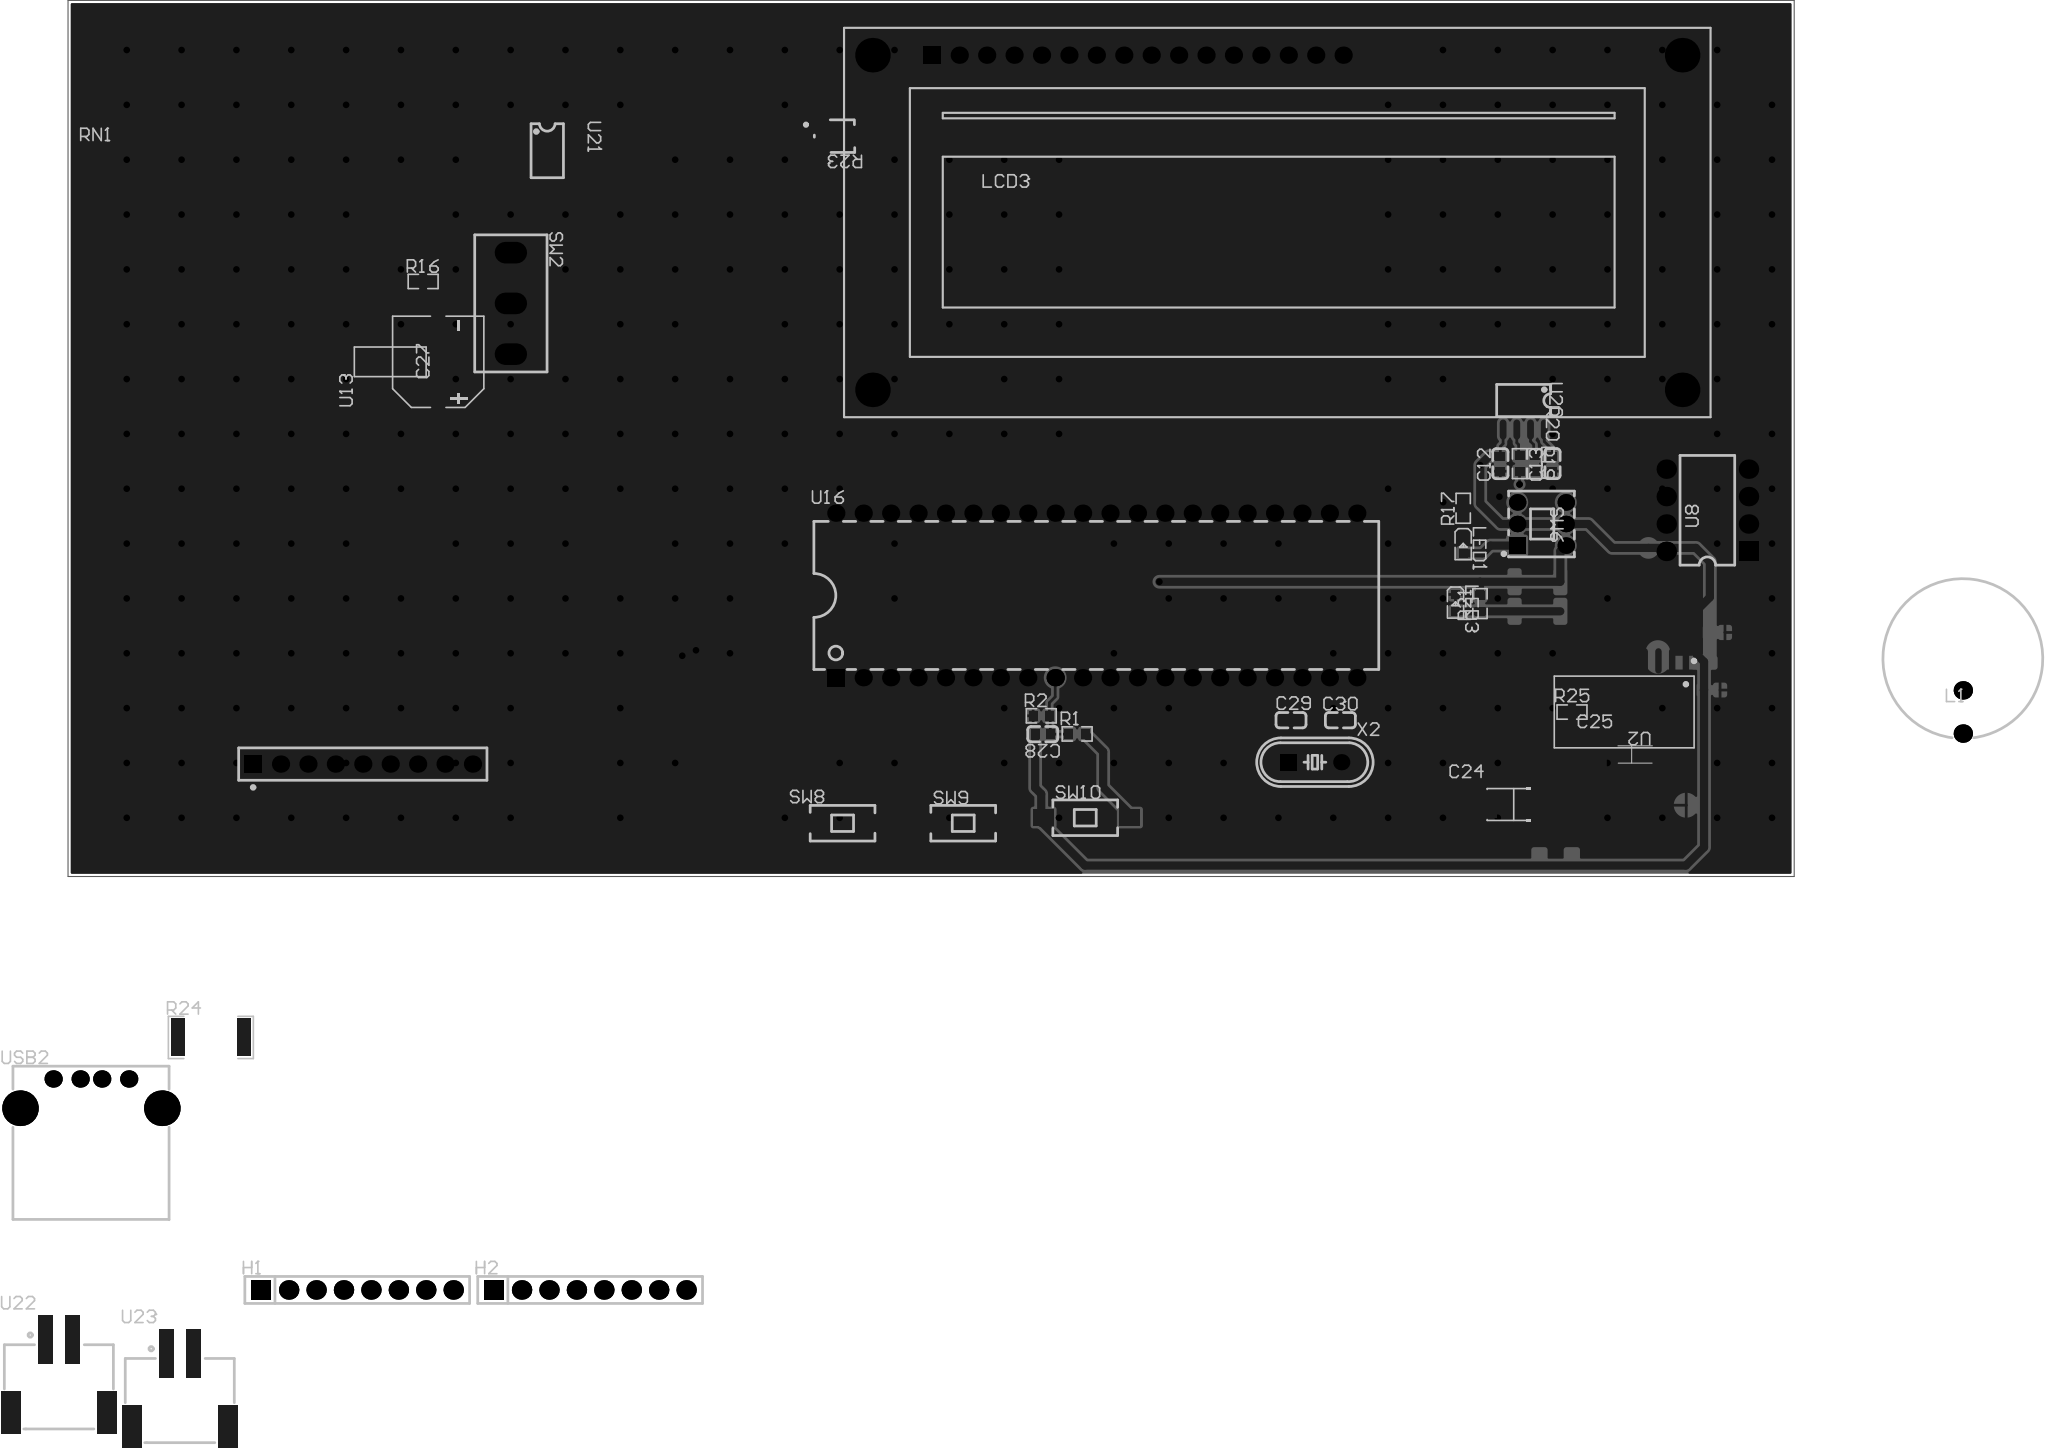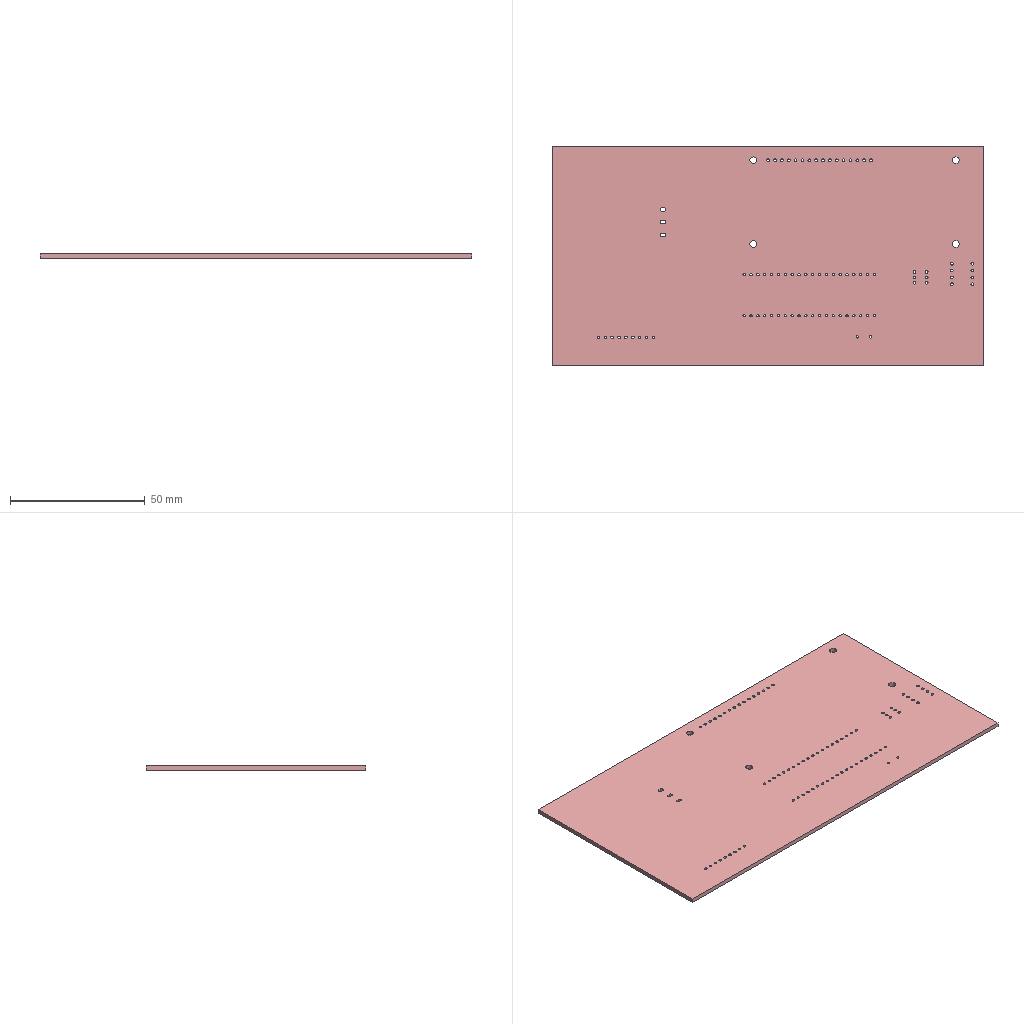Circuit board layout | Altium Designer | box 159.9 x 81.2 x 1.6 mm
Layer stack:
# Altium Designer layer stack of  (unit mm; dielectric type: 0 none, 1 core, 2 prepreg, 3 surface material)
index,name,kind,layer,copper_thickness_mm,dielectric_type,dielectric_thickness_mm,dielectric_material,dielectric_constant
0,Top Paste Mask Layer,other,,,,,,
1,Top Silkscreen Layer,other,,,,,,
2,Top Solder Mask Layer,dielectric,,,3,0.01,,3.3
3,Top Layer,copper,Top Layer,0.035,,,,
4,Dielectric1,dielectric,,,3,1.51,FR4,4.5
5,Bottom Layer,copper,Bottom Layer,0.035,,,,
6,Bottom Solder Mask Layer,dielectric,,,3,0.01,,3.3
7,Bottom Silkscreen Layer,other,,,,,,
8,Bottom Paste Mask Layer,other,,,,,,
# drill layer pairs: low layer,high layer
drill_pair,Top Layer,Bottom Layer
Part placement:
Designator,Comment,Layer,Footprint,Center-X(mm),Center-Y(mm),Rotation
R1,10K,TopLayer,R0603,175.821,142.302,0
R2,10K,TopLayer,R0603,172.499,143.979,0
R24,5Ω,TopLayer,R2512,95.58,114.184,0
H1,,TopLayer,HDR-TH_8P-P2.54-V-F-1,109.137,90.797,0
H2,,TopLayer,HDR-TH_8P-P2.54-V-F-1,130.711,90.797,0
U22,XH2.54-2PSMD,TopLayer,CONN-SMD_XH2.54-2PSMD,81.55,82.82,0
U23,XH2.54-2PSMD,TopLayer,CONN-SMD_XH2.54-2PSMD,92.75,81.55,0
U13,LT3092EST#TRPBF,TopLayer,SOT-223-4_L6.5-W3.5-P2.30-LS7.0-BR,112.195,176.769,90
C12,0.1uF,TopLayer,C0603,215.025,167.334,90
C13,0.1uF,TopLayer,C0603,219.851,167.337,90
U21,AD620ARZ-REEL7,TopLayer,SOIC-8_L5.0-W4.0-P1.27-LS6.0-BL,126.738,196.323,270
U16,STC89C52RC-40I-PDIP40,TopLayer,DIP-40_L52.0-W13.7-P2.54-LS15.2-BL,177.599,155.129,0
R16,100K,TopLayer,R0603,115.242,184.212,0
SW2,SS-12D10L5,TopLayer,SW-TH_SS-12D10L5,123.37,182.18,270
USB2,USB-231-ARY,TopLayer,USB-A-TH_USB-231-ARY,84.471,108.985,0
R17,1K,TopLayer,R0603,211.583,163.201,90
LED1,,TopLayer,LED_0603,211.576,159.829,270
LCD3,HS1602A,TopLayer,LCD1602,194.363,189.673,0
X2,11.059MHz,TopLayer,HC-49US_L11.5-W4.5-P4.88,197.848,139.681,0
LED3,,TopLayer,LED_0603,210.866,154.418,270
R21,1K,TopLayer,R0603,213.137,154.374,90
U20,CH340N,TopLayer,SOP-8_L4.9-W3.9-P1.27-LS6.0-BL,217.184,173.176,180
R19,100Ω,TopLayer,R0603,218.2,167.337,270
R20,100Ω,TopLayer,R0603,216.803,167.337,270
SW6,5.8 ZSGT,TopLayer,SW-TH_5.8ZSGT,218.835,161.746,270
SW8,TS-1101-C-W,TopLayer,SW-SMD_L6.0-W3.3-LS8.0,154.231,134.047,0
SW9,TS-1101-C-W,TopLayer,SW-SMD_L6.0-W3.3-LS8.0,165.407,134.047,0
C24,22uF,TopLayer,CAP-SMD_L3.5-W2.8-R-RD,215.628,135.763,0
C25,100nF,TopLayer,CASE-A_3216,227.51,140.397,0
U2,DAC0832LCWMX/NOPB,TopLayer,SOIC-20_L13.0-W7.6-P1.27-LS10.3-BL,226.494,144.334,180
U8,ADC0832CCN,TopLayer,DIP-8_L9.7-W6.4-P2.54-LS7.6-BL,234.202,163.016,90
RN1,1kΩ,TopLayer,RES-ARRAY-TH_9P-P2.54-D1.0,109.654,139.508,0
L1,22uH,TopLayer,IND-TH_BD14.7-2P-P4.00,257.863,144.334,0
R25,14kΩ,TopLayer,R0603,221.661,144.326,0
C27,100uF,TopLayer,CAP-SMD_BD8.1-L8.3-W8.3-LS9.3-FD,116.64,176.769,90
C28,47pF,TopLayer,C0603,172.633,142.28,180
C29,47pF,TopLayer,C0603,195.633,143.572,180
C30,10uF,TopLayer,C0603,200.205,143.572,0
SW10,TS-1101-C-W,TopLayer,SW-SMD_L6.0-W3.3-LS8.0,176.71,134.555,0
R23,10kΩ,TopLayer,RES-ADJ-SMD_3P-L3.0-W3.8-P1.75-BR,153.469,197.674,180
Pad and via stacks:
# Altium Designer via and pad stacks of  (unit mm). Each distinct definition once, with the count of objects using it.
# via: kind,start_layer,end_layer,hole_mm,diameter_mm,mode(0 simple;1 top-mid-bottom;2 full stack),diameter_per_layer,count,example_net
# pad: kind,layer,hole_mm,hole_type(0 round;1 square;2 slot),plating,top_size,top_shape(1 round;2 rect;3 octagon;9 rounded rect),mid_size,bottom_size,mode,footprint,size_per_layer,count,example
pad,Top Layer,0,0,plated,0.8065x0.864,2,0.8065x0.864,0.8065x0.864,0,R0603,,16,R1.2
pad,Top Layer,0,0,plated,1.282x3.456,2,1.282x3.456,1.282x3.456,0,R2512,,2,R24.2
pad,Top Layer,0,0,plated,1.3x4.5,2,1.3x4.5,1.3x4.5,0,CONN-SMD_XH2.54-2PSMD,,4,U22.1
pad,Top Layer,0,0,plated,1.8x3.9,2,1.8x3.9,1.8x3.9,0,CONN-SMD_XH2.54-2PSMD,,4,U22.3
pad,Top Layer,0,0,plated,2.47x0.98,2,2.47x0.98,2.47x0.98,0,SOT-223-4_L6.5-W3.5-P2.30-LS7.0-BR,,3,U13.1
pad,Top Layer,0,0,plated,2.47x3.6,2,2.47x3.6,2.47x3.6,0,SOT-223-4_L6.5-W3.5-P2.30-LS7.0-BR,,1,U13.4
pad,Top Layer,0,0,plated,0.8x0.9,2,0.8x0.9,0.8x0.9,0,C0603,,10,C12.2
pad,Top Layer,0,0,plated,0.5684x1.95,1,0.5684x1.95,0.5684x1.95,0,SOIC-8_L5.0-W4.0-P1.27-LS6.0-BL,,8,U21.1
pad,Top Layer,0,0,plated,0.8001x0.8001,2,0.8001x0.8001,0.8001x0.8001,0,LED_0603,,4,LED1.1
pad,Top Layer,0,0,plated,0.63x1.865,1,0.63x1.865,0.63x1.865,0,SOP-8_L4.9-W3.9-P1.27-LS6.0-BL,,8,U20.1
pad,Top Layer,0,0,plated,1.9x1.5,2,1.9x1.5,1.9x1.5,0,SW-SMD_L6.0-W3.3-LS8.0,,6,SW8.1
pad,Top Layer,0,0,plated,1.9x2.376,2,1.9x2.376,1.9x2.376,0,CAP-SMD_L3.5-W2.8-R-RD,,2,C24.1
pad,Top Layer,0,0,plated,1.5x1.359,2,1.5x1.359,1.5x1.359,0,CASE-A_3216,,2,C25.1
pad,Top Layer,0,0,plated,0.595x2.36,1,0.595x2.36,0.595x2.36,0,SOIC-20_L13.0-W7.6-P1.27-LS10.3-BL,,20,U2.1
pad,Top Layer,0,0,plated,3.56x1.12,2,3.56x1.12,3.56x1.12,0,CAP-SMD_BD8.1-L8.3-W8.3-LS9.3-FD,,2,C27.1
pad,Top Layer,0,0,plated,1.6x1.5,2,1.6x1.5,1.6x1.5,0,RES-ADJ-SMD_3P-L3.0-W3.8-P1.75-BR,,1,R23.2
pad,Top Layer,0,0,plated,1.2x1.2,2,1.2x1.2,1.2x1.2,0,RES-ADJ-SMD_3P-L3.0-W3.8-P1.75-BR,,2,R23.1
pad,Multi-Layer,1.2,0,plated,1.8x1.8,2,1.8x1.8,1.8x1.8,0,HDR-TH_8P-P2.54-V-F-1,,2,H1.1
pad,Multi-Layer,1.2,0,plated,1.8x1.8,1,1.8x1.8,1.8x1.8,0,HDR-TH_8P-P2.54-V-F-1,,14,H1.2
pad,Multi-Layer,0.889,0,plated,1.6x1.6,1,1.6x1.6,1.6x1.6,0,DIP-40_L52.0-W13.7-P2.54-LS15.2-BL,,39,U16.31
pad,Multi-Layer,0.889,0,plated,1.6x1.6,2,1.6x1.6,1.6x1.6,0,DIP-40_L52.0-W13.7-P2.54-LS15.2-BL,,1,U16.1
pad,Multi-Layer,1.3,2,plated,2x3,1,2x3,2x3,0,SW-TH_SS-12D10L5,,3,SW2.1
pad,Multi-Layer,1,0,plated,1.6x1.6,1,1.6x1.6,1.6x1.6,0,USB-A-TH_USB-231-ARY,,4,USB2.1
pad,Multi-Layer,2.5,0,plated,3.3x3.3,1,3.3x3.3,3.3x3.3,0,USB-A-TH_USB-231-ARY,,2,USB2.5
pad,Multi-Layer,1,0,plated,1.6x1.6,1,1.6x1.6,1.6x1.6,0,LCD1602,,15,LCD3.16
pad,Multi-Layer,1,0,plated,1.6x1.6,2,1.6x1.6,1.6x1.6,0,LCD1602,,1,LCD3.1
pad,Multi-Layer,2.5,2,plated,3.2x3.2,1,3.2x3.2,3.2x3.2,0,LCD1602,,4,LCD3.0
pad,Multi-Layer,0.9,0,plated,1.5x1.5,2,1.5x1.5,1.5x1.5,0,HC-49US_L11.5-W4.5-P4.88,,1,X2.1
pad,Multi-Layer,0.9,0,plated,1.5x1.5,1,1.5x1.5,1.5x1.5,0,HC-49US_L11.5-W4.5-P4.88,,1,X2.2
pad,Multi-Layer,1,0,plated,1.524x1.524,1,1.524x1.524,1.524x1.524,0,SW-TH_5.8ZSGT,,5,SW6.4
pad,Multi-Layer,1,0,plated,1.524x1.524,2,1.524x1.524,1.524x1.524,0,SW-TH_5.8ZSGT,,1,SW6.1
pad,Multi-Layer,1,0,plated,1.8x1.8,2,1.8x1.8,1.8x1.8,0,DIP-8_L9.7-W6.4-P2.54-LS7.6-BL,,1,U8.1
pad,Multi-Layer,1,0,plated,1.8x1.8,1,1.8x1.8,1.8x1.8,0,DIP-8_L9.7-W6.4-P2.54-LS7.6-BL,,7,U8.2
pad,Multi-Layer,1,0,plated,1.6x1.6,2,1.6x1.6,1.6x1.6,0,RES-ARRAY-TH_9P-P2.54-D1.0,,1,RN1.1
pad,Multi-Layer,1,0,plated,1.6x1.6,1,1.6x1.6,1.6x1.6,0,RES-ARRAY-TH_9P-P2.54-D1.0,,8,RN1.2
pad,Multi-Layer,1.1,0,plated,1.7x1.7,1,1.7x1.7,1.7x1.7,0,IND-TH_BD14.7-2P-P4.00,,2,L1.1
via,Top Layer,Bottom Layer,0.3048,0.61,0,,333,P3.1
Copper pours:
name,layer,net,type(0 solid;1 hatched;2 none)
Top Layer-GND,Top Layer,GND,0
Bottom Layer-GND,Bottom Layer,GND,0
Design rules, without the lines most boards share:
# Altium Designer design rules of  (exported by Altium Designer, unit mm)
# columns: name | kind | enabled | priority | scope1 | scope2 | descriptor | typed fields (field=value)
otherClearance | 52 | enabled | 1 | All | All | Hole To Hole Clearance (Gap=11.8mil) (All),(All) | gap=0.2997